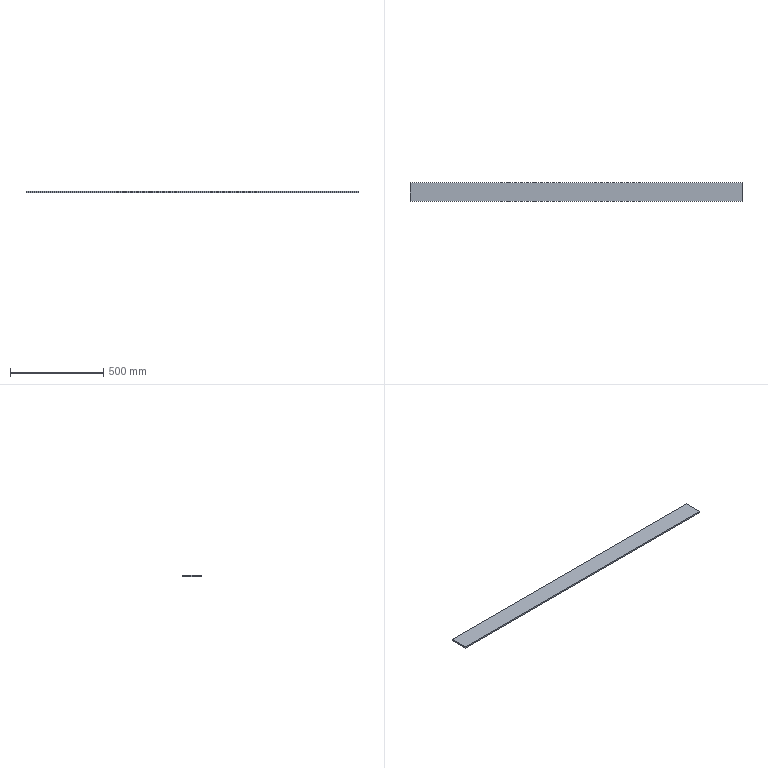Part | STEP file | Plate 1784X80X8_Default<As machined> | 1 solid | 6 faces | box 1784 x 100 x 8 mm | volume 1427200 mm3 | plane 6
STEP:
#1=CARTESIAN_POINT('',(0.,0.,0.));
#2=DIRECTION('',(0.,0.,1.));
#3=DIRECTION('',(1.,0.,0.));
#4=AXIS2_PLACEMENT_3D('',#1,#2,#3);
#5=CARTESIAN_POINT('',(892.,-50.,0.));
#6=VERTEX_POINT('',#5);
#7=CARTESIAN_POINT('',(892.,50.,0.));
#8=VERTEX_POINT('',#7);
#9=CARTESIAN_POINT('',(892.,50.,0.));
#10=DIRECTION('',(0.,1.,0.));
#11=VECTOR('',#10,1.);
#12=LINE('',#9,#11);
#13=CARTESIAN_POINT('',(892.,50.,8.));
#14=DIRECTION('',(-1.,0.,0.));
#15=DIRECTION('',(0.,-1.,0.));
#16=AXIS2_PLACEMENT_3D('',#13,#14,#15);
#17=PLANE('',#16);
#18=CARTESIAN_POINT('',(0.,-8.));
#19=DIRECTION('',(-1.,0.));
#20=VECTOR('',#19,1.);
#21=LINE('',#18,#20);
#22=(GEOMETRIC_REPRESENTATION_CONTEXT(2)PARAMETRIC_REPRESENTATION_CONTEXT()REPRESENTATION_CONTEXT('',''));
#23=DEFINITIONAL_REPRESENTATION('',(#21),#22);
#24=PCURVE('',#17,#23);
#25=CARTESIAN_POINT('',(0.,0.,0.));
#26=DIRECTION('',(0.,0.,1.));
#27=DIRECTION('',(1.,0.,0.));
#28=AXIS2_PLACEMENT_3D('',#25,#26,#27);
#29=PLANE('',#28);
#30=CARTESIAN_POINT('',(892.,50.));
#31=DIRECTION('',(0.,1.));
#32=VECTOR('',#31,1.);
#33=LINE('',#30,#32);
#34=(GEOMETRIC_REPRESENTATION_CONTEXT(2)PARAMETRIC_REPRESENTATION_CONTEXT()REPRESENTATION_CONTEXT('',''));
#35=DEFINITIONAL_REPRESENTATION('',(#33),#34);
#36=PCURVE('',#29,#35);
#37=SURFACE_CURVE('',#12,(#24,#36),.PCURVE_S1.);
#38=EDGE_CURVE('',#6,#8,#37,.T.);
#39=ORIENTED_EDGE('',*,*,#38,.T.);
#40=CARTESIAN_POINT('',(892.,50.,8.));
#41=VERTEX_POINT('',#40);
#42=CARTESIAN_POINT('',(892.,50.,8.));
#43=DIRECTION('',(0.,0.,-1.));
#44=VECTOR('',#43,1.);
#45=LINE('',#42,#44);
#46=CARTESIAN_POINT('',(0.,0.));
#47=DIRECTION('',(0.,-1.));
#48=VECTOR('',#47,1.);
#49=LINE('',#46,#48);
#50=(GEOMETRIC_REPRESENTATION_CONTEXT(2)PARAMETRIC_REPRESENTATION_CONTEXT()REPRESENTATION_CONTEXT('',''));
#51=DEFINITIONAL_REPRESENTATION('',(#49),#50);
#52=PCURVE('',#17,#51);
#53=CARTESIAN_POINT('',(-892.,50.,8.));
#54=DIRECTION('',(0.,-1.,0.));
#55=DIRECTION('',(0.,0.,-1.));
#56=AXIS2_PLACEMENT_3D('',#53,#54,#55);
#57=PLANE('',#56);
#58=CARTESIAN_POINT('',(0.,1784.));
#59=DIRECTION('',(1.,0.));
#60=VECTOR('',#59,1.);
#61=LINE('',#58,#60);
#62=(GEOMETRIC_REPRESENTATION_CONTEXT(2)PARAMETRIC_REPRESENTATION_CONTEXT()REPRESENTATION_CONTEXT('',''));
#63=DEFINITIONAL_REPRESENTATION('',(#61),#62);
#64=PCURVE('',#57,#63);
#65=SURFACE_CURVE('',#45,(#52,#64),.PCURVE_S1.);
#66=EDGE_CURVE('',#41,#8,#65,.T.);
#67=ORIENTED_EDGE('',*,*,#66,.F.);
#68=CARTESIAN_POINT('',(892.,-50.,8.));
#69=VERTEX_POINT('',#68);
#70=CARTESIAN_POINT('',(892.,50.,8.));
#71=DIRECTION('',(0.,1.,0.));
#72=VECTOR('',#71,1.);
#73=LINE('',#70,#72);
#74=CARTESIAN_POINT('',(0.,0.));
#75=DIRECTION('',(-1.,0.));
#76=VECTOR('',#75,1.);
#77=LINE('',#74,#76);
#78=(GEOMETRIC_REPRESENTATION_CONTEXT(2)PARAMETRIC_REPRESENTATION_CONTEXT()REPRESENTATION_CONTEXT('',''));
#79=DEFINITIONAL_REPRESENTATION('',(#77),#78);
#80=PCURVE('',#17,#79);
#81=CARTESIAN_POINT('',(0.,0.,8.));
#82=DIRECTION('',(0.,0.,1.));
#83=DIRECTION('',(1.,0.,0.));
#84=AXIS2_PLACEMENT_3D('',#81,#82,#83);
#85=PLANE('',#84);
#86=CARTESIAN_POINT('',(892.,50.));
#87=DIRECTION('',(0.,1.));
#88=VECTOR('',#87,1.);
#89=LINE('',#86,#88);
#90=(GEOMETRIC_REPRESENTATION_CONTEXT(2)PARAMETRIC_REPRESENTATION_CONTEXT()REPRESENTATION_CONTEXT('',''));
#91=DEFINITIONAL_REPRESENTATION('',(#89),#90);
#92=PCURVE('',#85,#91);
#93=SURFACE_CURVE('',#73,(#80,#92),.PCURVE_S1.);
#94=EDGE_CURVE('',#69,#41,#93,.T.);
#95=ORIENTED_EDGE('',*,*,#94,.F.);
#96=CARTESIAN_POINT('',(892.,-50.,8.));
#97=DIRECTION('',(0.,0.,-1.));
#98=VECTOR('',#97,1.);
#99=LINE('',#96,#98);
#100=CARTESIAN_POINT('',(100.,0.));
#101=DIRECTION('',(0.,-1.));
#102=VECTOR('',#101,1.);
#103=LINE('',#100,#102);
#104=(GEOMETRIC_REPRESENTATION_CONTEXT(2)PARAMETRIC_REPRESENTATION_CONTEXT()REPRESENTATION_CONTEXT('',''));
#105=DEFINITIONAL_REPRESENTATION('',(#103),#104);
#106=PCURVE('',#17,#105);
#107=CARTESIAN_POINT('',(-892.,-50.,8.));
#108=DIRECTION('',(0.,1.,0.));
#109=DIRECTION('',(0.,0.,1.));
#110=AXIS2_PLACEMENT_3D('',#107,#108,#109);
#111=PLANE('',#110);
#112=CARTESIAN_POINT('',(0.,1784.));
#113=DIRECTION('',(-1.,0.));
#114=VECTOR('',#113,1.);
#115=LINE('',#112,#114);
#116=(GEOMETRIC_REPRESENTATION_CONTEXT(2)PARAMETRIC_REPRESENTATION_CONTEXT()REPRESENTATION_CONTEXT('',''));
#117=DEFINITIONAL_REPRESENTATION('',(#115),#116);
#118=PCURVE('',#111,#117);
#119=SURFACE_CURVE('',#99,(#106,#118),.PCURVE_S1.);
#120=EDGE_CURVE('',#69,#6,#119,.T.);
#121=ORIENTED_EDGE('',*,*,#120,.T.);
#122=EDGE_LOOP('',(#39,#67,#95,#121));
#123=FACE_BOUND('',#122,.T.);
#124=ADVANCED_FACE('',(#123),#17,.F.);
#125=CARTESIAN_POINT('',(-892.,50.,0.));
#126=VERTEX_POINT('',#125);
#127=CARTESIAN_POINT('',(-892.,50.,0.));
#128=DIRECTION('',(-1.,0.,0.));
#129=VECTOR('',#128,1.);
#130=LINE('',#127,#129);
#131=CARTESIAN_POINT('',(8.,0.));
#132=DIRECTION('',(0.,-1.));
#133=VECTOR('',#132,1.);
#134=LINE('',#131,#133);
#135=(GEOMETRIC_REPRESENTATION_CONTEXT(2)PARAMETRIC_REPRESENTATION_CONTEXT()REPRESENTATION_CONTEXT('',''));
#136=DEFINITIONAL_REPRESENTATION('',(#134),#135);
#137=PCURVE('',#57,#136);
#138=CARTESIAN_POINT('',(-892.,50.));
#139=DIRECTION('',(-1.,0.));
#140=VECTOR('',#139,1.);
#141=LINE('',#138,#140);
#142=(GEOMETRIC_REPRESENTATION_CONTEXT(2)PARAMETRIC_REPRESENTATION_CONTEXT()REPRESENTATION_CONTEXT('',''));
#143=DEFINITIONAL_REPRESENTATION('',(#141),#142);
#144=PCURVE('',#29,#143);
#145=SURFACE_CURVE('',#130,(#137,#144),.PCURVE_S1.);
#146=EDGE_CURVE('',#8,#126,#145,.T.);
#147=ORIENTED_EDGE('',*,*,#146,.T.);
#148=CARTESIAN_POINT('',(-892.,50.,8.));
#149=VERTEX_POINT('',#148);
#150=CARTESIAN_POINT('',(-892.,50.,8.));
#151=DIRECTION('',(0.,0.,-1.));
#152=VECTOR('',#151,1.);
#153=LINE('',#150,#152);
#154=CARTESIAN_POINT('',(0.,0.));
#155=DIRECTION('',(1.,0.));
#156=VECTOR('',#155,1.);
#157=LINE('',#154,#156);
#158=(GEOMETRIC_REPRESENTATION_CONTEXT(2)PARAMETRIC_REPRESENTATION_CONTEXT()REPRESENTATION_CONTEXT('',''));
#159=DEFINITIONAL_REPRESENTATION('',(#157),#158);
#160=PCURVE('',#57,#159);
#161=CARTESIAN_POINT('',(-892.,50.,8.));
#162=DIRECTION('',(1.,0.,0.));
#163=DIRECTION('',(0.,1.,0.));
#164=AXIS2_PLACEMENT_3D('',#161,#162,#163);
#165=PLANE('',#164);
#166=CARTESIAN_POINT('',(0.,0.));
#167=DIRECTION('',(0.,-1.));
#168=VECTOR('',#167,1.);
#169=LINE('',#166,#168);
#170=(GEOMETRIC_REPRESENTATION_CONTEXT(2)PARAMETRIC_REPRESENTATION_CONTEXT()REPRESENTATION_CONTEXT('',''));
#171=DEFINITIONAL_REPRESENTATION('',(#169),#170);
#172=PCURVE('',#165,#171);
#173=SURFACE_CURVE('',#153,(#160,#172),.PCURVE_S1.);
#174=EDGE_CURVE('',#149,#126,#173,.T.);
#175=ORIENTED_EDGE('',*,*,#174,.F.);
#176=CARTESIAN_POINT('',(-892.,50.,8.));
#177=DIRECTION('',(-1.,0.,0.));
#178=VECTOR('',#177,1.);
#179=LINE('',#176,#178);
#180=CARTESIAN_POINT('',(0.,0.));
#181=DIRECTION('',(0.,-1.));
#182=VECTOR('',#181,1.);
#183=LINE('',#180,#182);
#184=(GEOMETRIC_REPRESENTATION_CONTEXT(2)PARAMETRIC_REPRESENTATION_CONTEXT()REPRESENTATION_CONTEXT('',''));
#185=DEFINITIONAL_REPRESENTATION('',(#183),#184);
#186=PCURVE('',#57,#185);
#187=CARTESIAN_POINT('',(-892.,50.));
#188=DIRECTION('',(-1.,0.));
#189=VECTOR('',#188,1.);
#190=LINE('',#187,#189);
#191=(GEOMETRIC_REPRESENTATION_CONTEXT(2)PARAMETRIC_REPRESENTATION_CONTEXT()REPRESENTATION_CONTEXT('',''));
#192=DEFINITIONAL_REPRESENTATION('',(#190),#191);
#193=PCURVE('',#85,#192);
#194=SURFACE_CURVE('',#179,(#186,#193),.PCURVE_S1.);
#195=EDGE_CURVE('',#41,#149,#194,.T.);
#196=ORIENTED_EDGE('',*,*,#195,.F.);
#197=ORIENTED_EDGE('',*,*,#66,.T.);
#198=EDGE_LOOP('',(#147,#175,#196,#197));
#199=FACE_BOUND('',#198,.T.);
#200=ADVANCED_FACE('',(#199),#57,.F.);
#201=CARTESIAN_POINT('',(-892.,-50.,0.));
#202=VERTEX_POINT('',#201);
#203=CARTESIAN_POINT('',(-892.,50.,0.));
#204=DIRECTION('',(0.,-1.,0.));
#205=VECTOR('',#204,1.);
#206=LINE('',#203,#205);
#207=CARTESIAN_POINT('',(0.,-8.));
#208=DIRECTION('',(-1.,0.));
#209=VECTOR('',#208,1.);
#210=LINE('',#207,#209);
#211=(GEOMETRIC_REPRESENTATION_CONTEXT(2)PARAMETRIC_REPRESENTATION_CONTEXT()REPRESENTATION_CONTEXT('',''));
#212=DEFINITIONAL_REPRESENTATION('',(#210),#211);
#213=PCURVE('',#165,#212);
#214=CARTESIAN_POINT('',(-892.,50.));
#215=DIRECTION('',(0.,-1.));
#216=VECTOR('',#215,1.);
#217=LINE('',#214,#216);
#218=(GEOMETRIC_REPRESENTATION_CONTEXT(2)PARAMETRIC_REPRESENTATION_CONTEXT()REPRESENTATION_CONTEXT('',''));
#219=DEFINITIONAL_REPRESENTATION('',(#217),#218);
#220=PCURVE('',#29,#219);
#221=SURFACE_CURVE('',#206,(#213,#220),.PCURVE_S1.);
#222=EDGE_CURVE('',#126,#202,#221,.T.);
#223=ORIENTED_EDGE('',*,*,#222,.T.);
#224=CARTESIAN_POINT('',(-892.,-50.,8.));
#225=VERTEX_POINT('',#224);
#226=CARTESIAN_POINT('',(-892.,-50.,8.));
#227=DIRECTION('',(0.,0.,-1.));
#228=VECTOR('',#227,1.);
#229=LINE('',#226,#228);
#230=CARTESIAN_POINT('',(-100.,0.));
#231=DIRECTION('',(0.,-1.));
#232=VECTOR('',#231,1.);
#233=LINE('',#230,#232);
#234=(GEOMETRIC_REPRESENTATION_CONTEXT(2)PARAMETRIC_REPRESENTATION_CONTEXT()REPRESENTATION_CONTEXT('',''));
#235=DEFINITIONAL_REPRESENTATION('',(#233),#234);
#236=PCURVE('',#165,#235);
#237=CARTESIAN_POINT('',(0.,0.));
#238=DIRECTION('',(-1.,0.));
#239=VECTOR('',#238,1.);
#240=LINE('',#237,#239);
#241=(GEOMETRIC_REPRESENTATION_CONTEXT(2)PARAMETRIC_REPRESENTATION_CONTEXT()REPRESENTATION_CONTEXT('',''));
#242=DEFINITIONAL_REPRESENTATION('',(#240),#241);
#243=PCURVE('',#111,#242);
#244=SURFACE_CURVE('',#229,(#236,#243),.PCURVE_S1.);
#245=EDGE_CURVE('',#225,#202,#244,.T.);
#246=ORIENTED_EDGE('',*,*,#245,.F.);
#247=CARTESIAN_POINT('',(-892.,50.,8.));
#248=DIRECTION('',(0.,-1.,0.));
#249=VECTOR('',#248,1.);
#250=LINE('',#247,#249);
#251=CARTESIAN_POINT('',(0.,0.));
#252=DIRECTION('',(-1.,0.));
#253=VECTOR('',#252,1.);
#254=LINE('',#251,#253);
#255=(GEOMETRIC_REPRESENTATION_CONTEXT(2)PARAMETRIC_REPRESENTATION_CONTEXT()REPRESENTATION_CONTEXT('',''));
#256=DEFINITIONAL_REPRESENTATION('',(#254),#255);
#257=PCURVE('',#165,#256);
#258=CARTESIAN_POINT('',(-892.,50.));
#259=DIRECTION('',(0.,-1.));
#260=VECTOR('',#259,1.);
#261=LINE('',#258,#260);
#262=(GEOMETRIC_REPRESENTATION_CONTEXT(2)PARAMETRIC_REPRESENTATION_CONTEXT()REPRESENTATION_CONTEXT('',''));
#263=DEFINITIONAL_REPRESENTATION('',(#261),#262);
#264=PCURVE('',#85,#263);
#265=SURFACE_CURVE('',#250,(#257,#264),.PCURVE_S1.);
#266=EDGE_CURVE('',#149,#225,#265,.T.);
#267=ORIENTED_EDGE('',*,*,#266,.F.);
#268=ORIENTED_EDGE('',*,*,#174,.T.);
#269=EDGE_LOOP('',(#223,#246,#267,#268));
#270=FACE_BOUND('',#269,.T.);
#271=ADVANCED_FACE('',(#270),#165,.F.);
#272=CARTESIAN_POINT('',(-892.,-50.,0.));
#273=DIRECTION('',(1.,0.,0.));
#274=VECTOR('',#273,1.);
#275=LINE('',#272,#274);
#276=CARTESIAN_POINT('',(-8.,0.));
#277=DIRECTION('',(0.,1.));
#278=VECTOR('',#277,1.);
#279=LINE('',#276,#278);
#280=(GEOMETRIC_REPRESENTATION_CONTEXT(2)PARAMETRIC_REPRESENTATION_CONTEXT()REPRESENTATION_CONTEXT('',''));
#281=DEFINITIONAL_REPRESENTATION('',(#279),#280);
#282=PCURVE('',#111,#281);
#283=CARTESIAN_POINT('',(-892.,-50.));
#284=DIRECTION('',(1.,0.));
#285=VECTOR('',#284,1.);
#286=LINE('',#283,#285);
#287=(GEOMETRIC_REPRESENTATION_CONTEXT(2)PARAMETRIC_REPRESENTATION_CONTEXT()REPRESENTATION_CONTEXT('',''));
#288=DEFINITIONAL_REPRESENTATION('',(#286),#287);
#289=PCURVE('',#29,#288);
#290=SURFACE_CURVE('',#275,(#282,#289),.PCURVE_S1.);
#291=EDGE_CURVE('',#202,#6,#290,.T.);
#292=ORIENTED_EDGE('',*,*,#291,.T.);
#293=ORIENTED_EDGE('',*,*,#120,.F.);
#294=CARTESIAN_POINT('',(-892.,-50.,8.));
#295=DIRECTION('',(1.,0.,0.));
#296=VECTOR('',#295,1.);
#297=LINE('',#294,#296);
#298=CARTESIAN_POINT('',(0.,0.));
#299=DIRECTION('',(0.,1.));
#300=VECTOR('',#299,1.);
#301=LINE('',#298,#300);
#302=(GEOMETRIC_REPRESENTATION_CONTEXT(2)PARAMETRIC_REPRESENTATION_CONTEXT()REPRESENTATION_CONTEXT('',''));
#303=DEFINITIONAL_REPRESENTATION('',(#301),#302);
#304=PCURVE('',#111,#303);
#305=CARTESIAN_POINT('',(-892.,-50.));
#306=DIRECTION('',(1.,0.));
#307=VECTOR('',#306,1.);
#308=LINE('',#305,#307);
#309=(GEOMETRIC_REPRESENTATION_CONTEXT(2)PARAMETRIC_REPRESENTATION_CONTEXT()REPRESENTATION_CONTEXT('',''));
#310=DEFINITIONAL_REPRESENTATION('',(#308),#309);
#311=PCURVE('',#85,#310);
#312=SURFACE_CURVE('',#297,(#304,#311),.PCURVE_S1.);
#313=EDGE_CURVE('',#225,#69,#312,.T.);
#314=ORIENTED_EDGE('',*,*,#313,.F.);
#315=ORIENTED_EDGE('',*,*,#245,.T.);
#316=EDGE_LOOP('',(#292,#293,#314,#315));
#317=FACE_BOUND('',#316,.T.);
#318=ADVANCED_FACE('',(#317),#111,.F.);
#319=ORIENTED_EDGE('',*,*,#94,.T.);
#320=ORIENTED_EDGE('',*,*,#195,.T.);
#321=ORIENTED_EDGE('',*,*,#266,.T.);
#322=ORIENTED_EDGE('',*,*,#313,.T.);
#323=EDGE_LOOP('',(#319,#320,#321,#322));
#324=FACE_BOUND('',#323,.T.);
#325=ADVANCED_FACE('',(#324),#85,.T.);
#326=ORIENTED_EDGE('',*,*,#38,.F.);
#327=ORIENTED_EDGE('',*,*,#291,.F.);
#328=ORIENTED_EDGE('',*,*,#222,.F.);
#329=ORIENTED_EDGE('',*,*,#146,.F.);
#330=EDGE_LOOP('',(#326,#327,#328,#329));
#331=FACE_BOUND('',#330,.T.);
#332=ADVANCED_FACE('',(#331),#29,.F.);
#333=CLOSED_SHELL('',(#124,#200,#271,#318,#325,#332));
#334=MANIFOLD_SOLID_BREP('',#333);
#335=(LENGTH_UNIT()NAMED_UNIT(*)SI_UNIT(.MILLI.,.METRE.));
#336=UNCERTAINTY_MEASURE_WITH_UNIT(LENGTH_MEASURE(0.0000001),#335,'','');
#337=(NAMED_UNIT(*)PLANE_ANGLE_UNIT()SI_UNIT($,.RADIAN.));
#338=(NAMED_UNIT(*)SI_UNIT($,.STERADIAN.)SOLID_ANGLE_UNIT());
#339=(GEOMETRIC_REPRESENTATION_CONTEXT(3)GLOBAL_UNCERTAINTY_ASSIGNED_CONTEXT((#336))GLOBAL_UNIT_ASSIGNED_CONTEXT((#335,#337,#338))REPRESENTATION_CONTEXT('',''));
#340=ADVANCED_BREP_SHAPE_REPRESENTATION('',(#4,#334),#339);